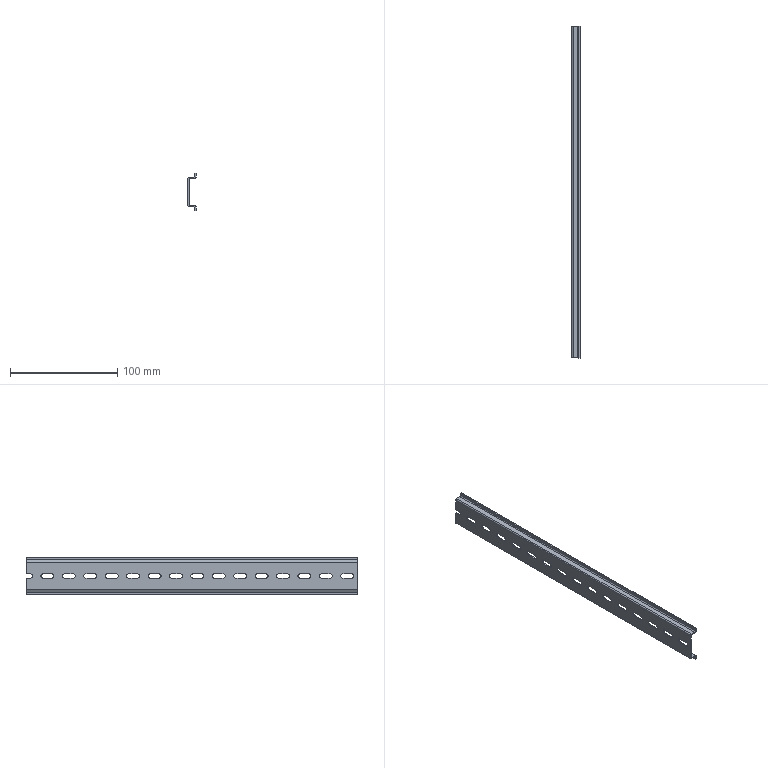Part | STEP file | c45-310 | 1 solid | 86 faces | box 7.5 x 310 x 35 mm | volume 14144 mm3 | plane 47 | cylinder 39 | commonest cylinder face diameters 4.2 x31 2 x8